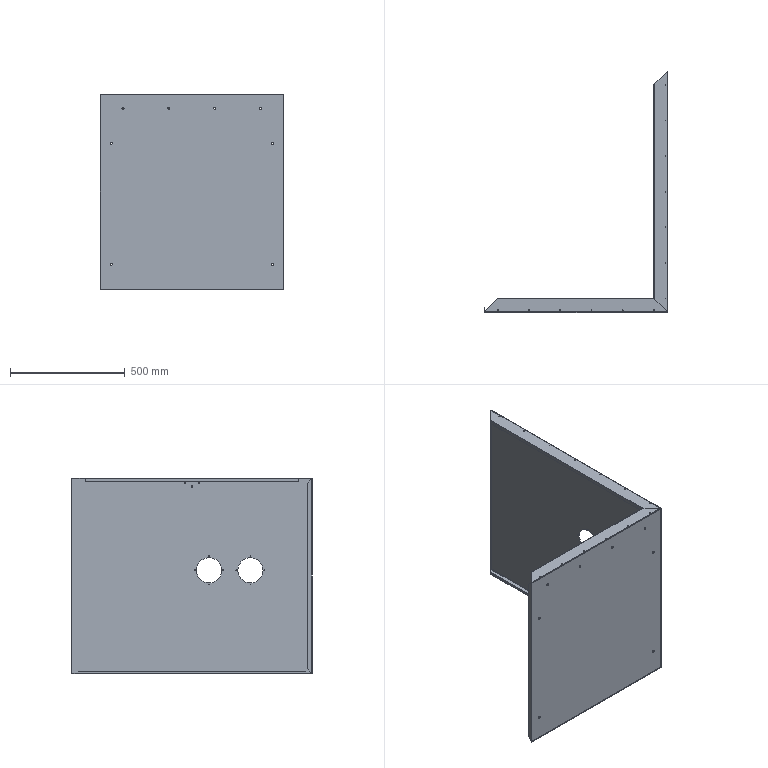Part | STEP file | HESS-408-70-15W-W-4-outer case side panel 4 | 1 solid | 166 faces | box 798.5 x 1049 x 850 mm | volume 2624739 mm3 | cylinder 88 | plane 72 | spline 6 | commonest cylinder face diameters 3.2 x26 3.5 x26 9 x16 0.2 x10 6 x6 110 x4